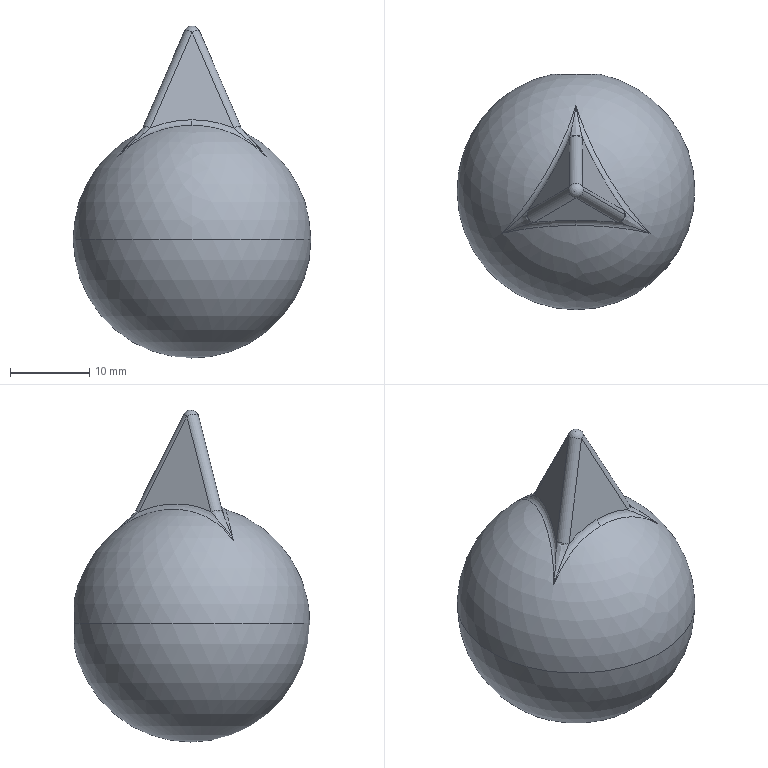Part | SolidWorks | features Fillet 2, Blend 1, ICE 1, Revolution 1 | 1 solid | 20 faces | box 30 x 29.697 x 41.877 mm | volume 14099 mm3 | cylinder 6 | torus 4 | plane 4 | sphere 3 | spline 3 | commonest cylinder face diameters 2 x4 6 x2
STEP:
#1=CARTESIAN_POINT('',(-3.,14.697,0.));
#2=VERTEX_POINT('',#1);
#3=CARTESIAN_POINT('',(0.,14.697,3.));
#4=VERTEX_POINT('',#3);
#5=CARTESIAN_POINT('',(0.,14.697,0.));
#6=DIRECTION('',(0.,1.,0.));
#7=DIRECTION('',(0.,0.,-1.));
#8=AXIS2_PLACEMENT_3D('',#5,#6,#7);
#9=CIRCLE('',#8,3.);
#10=EDGE_CURVE('',#2,#4,#9,.T.);
#11=ORIENTED_EDGE('',*,*,#10,.T.);
#12=CARTESIAN_POINT('',(0.,0.,3.));
#13=VERTEX_POINT('',#12);
#14=CARTESIAN_POINT('',(0.,26.,3.));
#15=DIRECTION('',(0.,-1.,0.));
#16=VECTOR('',#15,1000.);
#17=LINE('',#14,#16);
#18=EDGE_CURVE('',#4,#13,#17,.T.);
#19=ORIENTED_EDGE('',*,*,#18,.T.);
#20=CARTESIAN_POINT('',(0.,0.,-3.));
#21=VERTEX_POINT('',#20);
#22=CARTESIAN_POINT('',(0.,0.,0.));
#23=DIRECTION('',(0.,1.,0.));
#24=DIRECTION('',(0.,0.,1.));
#25=AXIS2_PLACEMENT_3D('',#22,#23,#24);
#26=CIRCLE('',#25,3.);
#27=EDGE_CURVE('',#21,#13,#26,.T.);
#28=ORIENTED_EDGE('',*,*,#27,.F.);
#29=CARTESIAN_POINT('',(0.,14.697,-3.));
#30=VERTEX_POINT('',#29);
#31=CARTESIAN_POINT('',(0.,26.,-3.));
#32=DIRECTION('',(0.,-1.,0.));
#33=VECTOR('',#32,1000.);
#34=LINE('',#31,#33);
#35=EDGE_CURVE('',#30,#21,#34,.T.);
#36=ORIENTED_EDGE('',*,*,#35,.F.);
#37=CARTESIAN_POINT('',(0.,14.697,0.));
#38=DIRECTION('',(0.,1.,0.));
#39=DIRECTION('',(0.,0.,-1.));
#40=AXIS2_PLACEMENT_3D('',#37,#38,#39);
#41=CIRCLE('',#40,3.);
#42=EDGE_CURVE('',#30,#2,#41,.T.);
#43=ORIENTED_EDGE('',*,*,#42,.T.);
#44=EDGE_LOOP('',(#11,#19,#28,#36,#43));
#45=FACE_OUTER_BOUND('',#44,.T.);
#46=CARTESIAN_POINT('',(0.,26.,0.));
#47=DIRECTION('',(0.,-1.,0.));
#48=DIRECTION('',(0.,0.,-1.));
#49=AXIS2_PLACEMENT_3D('',#46,#47,#48);
#50=CYLINDRICAL_SURFACE('',#49,3.);
#51=ADVANCED_FACE('',(#45),#50,.F.);
#52=CARTESIAN_POINT('',(5.23,-3.989,14.042));
#53=VERTEX_POINT('',#52);
#54=CARTESIAN_POINT('',(6.147,-3.019,14.197));
#55=VERTEX_POINT('',#54);
#56=CARTESIAN_POINT('',(5.23,-3.019,13.8));
#57=DIRECTION('',(-0.3873,0.2236,0.8944));
#58=DIRECTION('',(0.9177,0.,0.3974));
#59=AXIS2_PLACEMENT_3D('',#56,#57,#58);
#60=CIRCLE('',#59,1.);
#61=EDGE_CURVE('',#53,#55,#60,.T.);
#62=ORIENTED_EDGE('',*,*,#61,.T.);
#63=CARTESIAN_POINT('',(0.9177,0.,26.274));
#64=VERTEX_POINT('',#63);
#65=CARTESIAN_POINT('',(9.882,-5.175,5.573));
#66=DIRECTION('',(-0.3873,0.2236,0.8944));
#67=VECTOR('',#66,1000.);
#68=LINE('',#65,#67);
#69=EDGE_CURVE('',#55,#64,#68,.T.);
#70=ORIENTED_EDGE('',*,*,#69,.T.);
#71=CARTESIAN_POINT('',(0.,-0.9701,26.119));
#72=VERTEX_POINT('',#71);
#73=CARTESIAN_POINT('',(0.,0.,25.877));
#74=DIRECTION('',(-0.3873,0.2236,0.8944));
#75=DIRECTION('',(0.9177,0.,0.3974));
#76=AXIS2_PLACEMENT_3D('',#73,#74,#75);
#77=CIRCLE('',#76,1.);
#78=EDGE_CURVE('',#72,#64,#77,.T.);
#79=ORIENTED_EDGE('',*,*,#78,.F.);
#80=CARTESIAN_POINT('',(8.964,-6.146,5.418));
#81=DIRECTION('',(-0.3873,0.2236,0.8944));
#82=VECTOR('',#81,1000.);
#83=LINE('',#80,#82);
#84=EDGE_CURVE('',#53,#72,#83,.T.);
#85=ORIENTED_EDGE('',*,*,#84,.F.);
#86=EDGE_LOOP('',(#62,#70,#79,#85));
#87=FACE_OUTER_BOUND('',#86,.T.);
#88=CARTESIAN_POINT('',(8.964,-5.175,5.175));
#89=DIRECTION('',(-0.3873,0.2236,0.8944));
#90=DIRECTION('',(0.9177,0.,0.3974));
#91=AXIS2_PLACEMENT_3D('',#88,#89,#90);
#92=CYLINDRICAL_SURFACE('',#91,1.);
#93=ADVANCED_FACE('',(#87),#92,.T.);
#94=CARTESIAN_POINT('',(0.,-3.738,15.049));
#95=VERTEX_POINT('',#94);
#96=CARTESIAN_POINT('',(0.,-7.059,1.765));
#97=DIRECTION('',(0.,0.9701,-0.2425));
#98=DIRECTION('',(0.,0.2425,0.9701));
#99=AXIS2_PLACEMENT_3D('',#96,#97,#98);
#100=CIRCLE('',#99,13.693);
#101=EDGE_CURVE('',#95,#53,#100,.T.);
#102=ORIENTED_EDGE('',*,*,#101,.F.);
#103=CARTESIAN_POINT('',(0.,-4.414,14.336));
#104=VERTEX_POINT('',#103);
#105=CARTESIAN_POINT('',(0.,-4.708,15.292));
#106=DIRECTION('',(-1.,0.,0.));
#107=DIRECTION('',(0.,-1.,0.));
#108=AXIS2_PLACEMENT_3D('',#105,#106,#107);
#109=CIRCLE('',#108,1.);
#110=EDGE_CURVE('',#95,#104,#109,.T.);
#111=ORIENTED_EDGE('',*,*,#110,.T.);
#112=CARTESIAN_POINT('',(9.336,-5.39,10.43));
#113=VERTEX_POINT('',#112);
#114=CARTESIAN_POINT('',(0.,-7.527,1.882));
#115=DIRECTION('',(0.,-0.9701,0.2425));
#116=DIRECTION('',(0.,0.2425,0.9701));
#117=AXIS2_PLACEMENT_3D('',#114,#115,#116);
#118=CIRCLE('',#117,12.837);
#119=EDGE_CURVE('',#113,#104,#118,.T.);
#120=ORIENTED_EDGE('',*,*,#119,.F.);
#121=CARTESIAN_POINT('',(9.336,-5.39,10.43));
#122=CARTESIAN_POINT('',(8.724,-5.147,11.103));
#123=CARTESIAN_POINT('',(8.051,-4.9,11.718));
#124=CARTESIAN_POINT('',(6.993,-4.539,12.584));
#125=CARTESIAN_POINT('',(6.633,-4.42,12.863));
#126=CARTESIAN_POINT('',(6.092,-4.248,13.285));
#127=CARTESIAN_POINT('',(5.912,-4.192,13.426));
#128=CARTESIAN_POINT('',(5.56,-4.085,13.719));
#129=CARTESIAN_POINT('',(5.385,-4.033,13.87));
#130=CARTESIAN_POINT('',(5.23,-3.989,14.042));
#131=B_SPLINE_CURVE_WITH_KNOTS('',3,(#121,#122,#123,#124,#125,#126,#127,#128,#129,#130),.UNSPECIFIED.,.F.,.F.,(4,2,2,2,4),(-0.0000199,0.002804,0.004216,0.004922,0.005628),.UNSPECIFIED.);
#132=EDGE_CURVE('',#113,#53,#131,.T.);
#133=ORIENTED_EDGE('',*,*,#132,.T.);
#134=EDGE_LOOP('',(#102,#111,#120,#133));
#135=FACE_OUTER_BOUND('',#134,.T.);
#136=CARTESIAN_POINT('',(0.,-8.029,2.007));
#137=DIRECTION('',(0.,0.9701,-0.2425));
#138=DIRECTION('',(0.,0.2425,0.9701));
#139=AXIS2_PLACEMENT_3D('',#136,#137,#138);
#140=TOROIDAL_SURFACE('',#139,13.693,1.);
#141=ADVANCED_FACE('',(#135),#140,.F.);
#142=CARTESIAN_POINT('',(0.,-15.,0.));
#143=VERTEX_POINT('',#142);
#144=CARTESIAN_POINT('',(3.,14.697,0.));
#145=VERTEX_POINT('',#144);
#146=CARTESIAN_POINT('',(0.,0.,0.));
#147=DIRECTION('',(0.,0.,1.));
#148=DIRECTION('',(1.,0.,0.));
#149=AXIS2_PLACEMENT_3D('',#146,#147,#148);
#150=CIRCLE('',#149,15.);
#151=EDGE_CURVE('',#143,#145,#150,.T.);
#152=ORIENTED_EDGE('',*,*,#151,.F.);
#153=CARTESIAN_POINT('',(0.,0.,0.));
#154=DIRECTION('',(0.,0.,-1.));
#155=DIRECTION('',(-1.,0.,0.));
#156=AXIS2_PLACEMENT_3D('',#153,#154,#155);
#157=CIRCLE('',#156,15.);
#158=EDGE_CURVE('',#143,#2,#157,.T.);
#159=ORIENTED_EDGE('',*,*,#158,.T.);
#160=ORIENTED_EDGE('',*,*,#42,.F.);
#161=CARTESIAN_POINT('',(0.,14.697,0.));
#162=DIRECTION('',(0.,1.,0.));
#163=DIRECTION('',(0.,0.,-1.));
#164=AXIS2_PLACEMENT_3D('',#161,#162,#163);
#165=CIRCLE('',#164,3.);
#166=EDGE_CURVE('',#145,#30,#165,.T.);
#167=ORIENTED_EDGE('',*,*,#166,.F.);
#168=EDGE_LOOP('',(#152,#159,#160,#167));
#169=FACE_OUTER_BOUND('',#168,.T.);
#170=CARTESIAN_POINT('',(0.,0.,0.));
#171=DIRECTION('',(0.,0.,-1.));
#172=DIRECTION('',(1.,0.,0.));
#173=AXIS2_PLACEMENT_3D('',#170,#171,#172);
#174=SPHERICAL_SURFACE('',#173,15.);
#175=ADVANCED_FACE('',(#169),#174,.T.);
#176=ORIENTED_EDGE('',*,*,#158,.F.);
#177=ORIENTED_EDGE('',*,*,#151,.T.);
#178=CARTESIAN_POINT('',(0.,14.697,0.));
#179=DIRECTION('',(0.,1.,0.));
#180=DIRECTION('',(0.,0.,-1.));
#181=AXIS2_PLACEMENT_3D('',#178,#179,#180);
#182=CIRCLE('',#181,3.);
#183=EDGE_CURVE('',#4,#145,#182,.T.);
#184=ORIENTED_EDGE('',*,*,#183,.F.);
#185=ORIENTED_EDGE('',*,*,#10,.F.);
#186=EDGE_LOOP('',(#176,#177,#184,#185));
#187=FACE_OUTER_BOUND('',#186,.T.);
#188=CARTESIAN_POINT('',(-9.336,-5.39,10.43));
#189=VERTEX_POINT('',#188);
#190=CARTESIAN_POINT('',(0.,10.78,10.43));
#191=VERTEX_POINT('',#190);
#192=CARTESIAN_POINT('',(-6.519,3.764,1.882));
#193=DIRECTION('',(-0.8402,0.4851,0.2425));
#194=DIRECTION('',(0.5,0.866,0.));
#195=AXIS2_PLACEMENT_3D('',#192,#193,#194);
#196=CIRCLE('',#195,12.837);
#197=EDGE_CURVE('',#189,#191,#196,.T.);
#198=ORIENTED_EDGE('',*,*,#197,.T.);
#199=CARTESIAN_POINT('',(6.519,3.764,1.882));
#200=DIRECTION('',(0.8402,0.4851,0.2425));
#201=DIRECTION('',(0.5,-0.866,0.));
#202=AXIS2_PLACEMENT_3D('',#199,#200,#201);
#203=CIRCLE('',#202,12.837);
#204=EDGE_CURVE('',#191,#113,#203,.T.);
#205=ORIENTED_EDGE('',*,*,#204,.T.);
#206=ORIENTED_EDGE('',*,*,#119,.T.);
#207=CARTESIAN_POINT('',(0.,-7.527,1.882));
#208=DIRECTION('',(0.,-0.9701,0.2425));
#209=DIRECTION('',(0.,0.2425,0.9701));
#210=AXIS2_PLACEMENT_3D('',#207,#208,#209);
#211=CIRCLE('',#210,12.837);
#212=EDGE_CURVE('',#104,#189,#211,.T.);
#213=ORIENTED_EDGE('',*,*,#212,.T.);
#214=EDGE_LOOP('',(#198,#205,#206,#213));
#215=FACE_BOUND('',#214,.T.);
#216=CARTESIAN_POINT('',(0.,0.,0.));
#217=DIRECTION('',(0.,0.,-1.));
#218=DIRECTION('',(1.,0.,0.));
#219=AXIS2_PLACEMENT_3D('',#216,#217,#218);
#220=SPHERICAL_SURFACE('',#219,15.);
#221=ADVANCED_FACE('',(#187,#215),#220,.T.);
#222=ORIENTED_EDGE('',*,*,#84,.T.);
#223=CARTESIAN_POINT('',(-5.23,-3.989,14.042));
#224=VERTEX_POINT('',#223);
#225=CARTESIAN_POINT('',(-8.964,-6.146,5.418));
#226=DIRECTION('',(-0.3873,-0.2236,-0.8944));
#227=VECTOR('',#226,1000.);
#228=LINE('',#225,#227);
#229=EDGE_CURVE('',#72,#224,#228,.T.);
#230=ORIENTED_EDGE('',*,*,#229,.T.);
#231=CARTESIAN_POINT('',(0.,-7.059,1.765));
#232=DIRECTION('',(0.,0.9701,-0.2425));
#233=DIRECTION('',(0.,0.2425,0.9701));
#234=AXIS2_PLACEMENT_3D('',#231,#232,#233);
#235=CIRCLE('',#234,13.693);
#236=EDGE_CURVE('',#224,#95,#235,.T.);
#237=ORIENTED_EDGE('',*,*,#236,.T.);
#238=ORIENTED_EDGE('',*,*,#101,.T.);
#239=EDGE_LOOP('',(#222,#230,#237,#238));
#240=FACE_OUTER_BOUND('',#239,.T.);
#241=CARTESIAN_POINT('',(0.,-7.059,1.765));
#242=DIRECTION('',(0.,0.9701,-0.2425));
#243=DIRECTION('',(0.,0.2425,0.9701));
#244=AXIS2_PLACEMENT_3D('',#241,#242,#243);
#245=PLANE('',#244);
#246=ADVANCED_FACE('',(#240),#245,.F.);
#247=CARTESIAN_POINT('',(-0.8402,6.524,14.042));
#248=VERTEX_POINT('',#247);
#249=CARTESIAN_POINT('',(-6.07,-2.534,14.042));
#250=VERTEX_POINT('',#249);
#251=CARTESIAN_POINT('',(-6.113,3.529,1.765));
#252=DIRECTION('',(0.8402,-0.4851,-0.2425));
#253=DIRECTION('',(0.5,0.866,0.));
#254=AXIS2_PLACEMENT_3D('',#251,#252,#253);
#255=CIRCLE('',#254,13.693);
#256=EDGE_CURVE('',#248,#250,#255,.T.);
#257=ORIENTED_EDGE('',*,*,#256,.T.);
#258=CARTESIAN_POINT('',(-0.8402,0.4851,26.119));
#259=VERTEX_POINT('',#258);
#260=CARTESIAN_POINT('',(-9.804,-4.69,5.418));
#261=DIRECTION('',(0.3873,0.2236,0.8944));
#262=VECTOR('',#261,1000.);
#263=LINE('',#260,#262);
#264=EDGE_CURVE('',#250,#259,#263,.T.);
#265=ORIENTED_EDGE('',*,*,#264,.T.);
#266=CARTESIAN_POINT('',(-0.8402,10.836,5.418));
#267=DIRECTION('',(0.,0.4472,-0.8944));
#268=VECTOR('',#267,1000.);
#269=LINE('',#266,#268);
#270=EDGE_CURVE('',#259,#248,#269,.T.);
#271=ORIENTED_EDGE('',*,*,#270,.T.);
#272=EDGE_LOOP('',(#257,#265,#271));
#273=FACE_OUTER_BOUND('',#272,.T.);
#274=CARTESIAN_POINT('',(-6.113,3.529,1.765));
#275=DIRECTION('',(0.8402,-0.4851,-0.2425));
#276=DIRECTION('',(0.5,0.866,0.));
#277=AXIS2_PLACEMENT_3D('',#274,#275,#276);
#278=PLANE('',#277);
#279=ADVANCED_FACE('',(#273),#278,.F.);
#280=CARTESIAN_POINT('',(0.8402,6.524,14.042));
#281=VERTEX_POINT('',#280);
#282=CARTESIAN_POINT('',(0.8402,0.4851,26.119));
#283=VERTEX_POINT('',#282);
#284=CARTESIAN_POINT('',(0.8402,10.836,5.418));
#285=DIRECTION('',(0.,-0.4472,0.8944));
#286=VECTOR('',#285,1000.);
#287=LINE('',#284,#286);
#288=EDGE_CURVE('',#281,#283,#287,.T.);
#289=ORIENTED_EDGE('',*,*,#288,.T.);
#290=CARTESIAN_POINT('',(6.07,-2.534,14.042));
#291=VERTEX_POINT('',#290);
#292=CARTESIAN_POINT('',(9.804,-4.69,5.418));
#293=DIRECTION('',(0.3873,-0.2236,-0.8944));
#294=VECTOR('',#293,1000.);
#295=LINE('',#292,#294);
#296=EDGE_CURVE('',#283,#291,#295,.T.);
#297=ORIENTED_EDGE('',*,*,#296,.T.);
#298=CARTESIAN_POINT('',(6.113,3.529,1.765));
#299=DIRECTION('',(-0.8402,-0.4851,-0.2425));
#300=DIRECTION('',(0.5,-0.866,0.));
#301=AXIS2_PLACEMENT_3D('',#298,#299,#300);
#302=CIRCLE('',#301,13.693);
#303=EDGE_CURVE('',#291,#281,#302,.T.);
#304=ORIENTED_EDGE('',*,*,#303,.T.);
#305=EDGE_LOOP('',(#289,#297,#304));
#306=FACE_OUTER_BOUND('',#305,.T.);
#307=CARTESIAN_POINT('',(6.113,3.529,1.765));
#308=DIRECTION('',(-0.8402,-0.4851,-0.2425));
#309=DIRECTION('',(0.5,-0.866,0.));
#310=AXIS2_PLACEMENT_3D('',#307,#308,#309);
#311=PLANE('',#310);
#312=ADVANCED_FACE('',(#306),#311,.F.);
#313=ORIENTED_EDGE('',*,*,#110,.F.);
#314=ORIENTED_EDGE('',*,*,#236,.F.);
#315=CARTESIAN_POINT('',(-5.23,-3.989,14.042));
#316=CARTESIAN_POINT('',(-5.385,-4.033,13.87));
#317=CARTESIAN_POINT('',(-5.56,-4.085,13.719));
#318=CARTESIAN_POINT('',(-5.912,-4.192,13.426));
#319=CARTESIAN_POINT('',(-6.092,-4.248,13.285));
#320=CARTESIAN_POINT('',(-6.633,-4.42,12.863));
#321=CARTESIAN_POINT('',(-6.993,-4.539,12.584));
#322=CARTESIAN_POINT('',(-8.051,-4.9,11.718));
#323=CARTESIAN_POINT('',(-8.723,-5.147,11.104));
#324=CARTESIAN_POINT('',(-9.336,-5.39,10.43));
#325=B_SPLINE_CURVE_WITH_KNOTS('',3,(#315,#316,#317,#318,#319,#320,#321,#322,#323,#324),.UNSPECIFIED.,.F.,.F.,(4,2,2,2,4),(0.,0.0007073,0.001415,0.002829,0.005658),.UNSPECIFIED.);
#326=EDGE_CURVE('',#224,#189,#325,.T.);
#327=ORIENTED_EDGE('',*,*,#326,.T.);
#328=ORIENTED_EDGE('',*,*,#212,.F.);
#329=EDGE_LOOP('',(#313,#314,#327,#328));
#330=FACE_OUTER_BOUND('',#329,.T.);
#331=CARTESIAN_POINT('',(0.,-8.029,2.007));
#332=DIRECTION('',(0.,0.9701,-0.2425));
#333=DIRECTION('',(0.,0.2425,0.9701));
#334=AXIS2_PLACEMENT_3D('',#331,#332,#333);
#335=TOROIDAL_SURFACE('',#334,13.693,1.);
#336=ADVANCED_FACE('',(#330),#335,.F.);
#337=ORIENTED_EDGE('',*,*,#197,.F.);
#338=CARTESIAN_POINT('',(-9.336,-5.39,10.43));
#339=CARTESIAN_POINT('',(-8.82,-4.982,11.103));
#340=CARTESIAN_POINT('',(-8.269,-4.522,11.718));
#341=CARTESIAN_POINT('',(-7.428,-3.787,12.584));
#342=CARTESIAN_POINT('',(-7.144,-3.534,12.863));
#343=CARTESIAN_POINT('',(-6.725,-3.152,13.285));
#344=CARTESIAN_POINT('',(-6.587,-3.024,13.426));
#345=CARTESIAN_POINT('',(-6.317,-2.773,13.719));
#346=CARTESIAN_POINT('',(-6.185,-2.647,13.87));
#347=CARTESIAN_POINT('',(-6.07,-2.534,14.042));
#348=B_SPLINE_CURVE_WITH_KNOTS('',3,(#338,#339,#340,#341,#342,#343,#344,#345,#346,#347),.UNSPECIFIED.,.F.,.F.,(4,2,2,2,4),(-0.00002565,0.002798,0.00421,0.004916,0.005622),.UNSPECIFIED.);
#349=EDGE_CURVE('',#189,#250,#348,.T.);
#350=ORIENTED_EDGE('',*,*,#349,.T.);
#351=ORIENTED_EDGE('',*,*,#256,.F.);
#352=CARTESIAN_POINT('',(-0.8402,6.524,14.042));
#353=CARTESIAN_POINT('',(-0.7998,6.68,13.87));
#354=CARTESIAN_POINT('',(-0.7574,6.857,13.719));
#355=CARTESIAN_POINT('',(-0.6741,7.216,13.426));
#356=CARTESIAN_POINT('',(-0.6328,7.4,13.285));
#357=CARTESIAN_POINT('',(-0.5114,7.954,12.863));
#358=CARTESIAN_POINT('',(-0.4341,8.326,12.584));
#359=CARTESIAN_POINT('',(-0.218,9.423,11.718));
#360=CARTESIAN_POINT('',(-0.09559,10.128,11.104));
#361=CARTESIAN_POINT('',(0.,10.78,10.43));
#362=B_SPLINE_CURVE_WITH_KNOTS('',3,(#352,#353,#354,#355,#356,#357,#358,#359,#360,#361),.UNSPECIFIED.,.F.,.F.,(4,2,2,2,4),(0.,0.0007073,0.001415,0.002829,0.005658),.UNSPECIFIED.);
#363=EDGE_CURVE('',#248,#191,#362,.T.);
#364=ORIENTED_EDGE('',*,*,#363,.T.);
#365=EDGE_LOOP('',(#337,#350,#351,#364));
#366=FACE_OUTER_BOUND('',#365,.T.);
#367=CARTESIAN_POINT('',(-6.953,4.014,2.007));
#368=DIRECTION('',(0.8402,-0.4851,-0.2425));
#369=DIRECTION('',(0.5,0.866,0.));
#370=AXIS2_PLACEMENT_3D('',#367,#368,#369);
#371=TOROIDAL_SURFACE('',#370,13.693,1.);
#372=ADVANCED_FACE('',(#366),#371,.F.);
#373=ORIENTED_EDGE('',*,*,#303,.F.);
#374=CARTESIAN_POINT('',(6.07,-2.534,14.042));
#375=CARTESIAN_POINT('',(6.185,-2.647,13.87));
#376=CARTESIAN_POINT('',(6.317,-2.773,13.719));
#377=CARTESIAN_POINT('',(6.587,-3.024,13.426));
#378=CARTESIAN_POINT('',(6.725,-3.152,13.285));
#379=CARTESIAN_POINT('',(7.144,-3.534,12.863));
#380=CARTESIAN_POINT('',(7.428,-3.787,12.584));
#381=CARTESIAN_POINT('',(8.269,-4.522,11.718));
#382=CARTESIAN_POINT('',(8.819,-4.981,11.104));
#383=CARTESIAN_POINT('',(9.336,-5.39,10.43));
#384=B_SPLINE_CURVE_WITH_KNOTS('',3,(#374,#375,#376,#377,#378,#379,#380,#381,#382,#383),.UNSPECIFIED.,.F.,.F.,(4,2,2,2,4),(0.,0.0007073,0.001415,0.002829,0.005658),.UNSPECIFIED.);
#385=EDGE_CURVE('',#291,#113,#384,.T.);
#386=ORIENTED_EDGE('',*,*,#385,.T.);
#387=ORIENTED_EDGE('',*,*,#204,.F.);
#388=CARTESIAN_POINT('',(0.,10.78,10.43));
#389=CARTESIAN_POINT('',(0.09546,10.129,11.103));
#390=CARTESIAN_POINT('',(0.218,9.423,11.718));
#391=CARTESIAN_POINT('',(0.4341,8.326,12.584));
#392=CARTESIAN_POINT('',(0.5114,7.954,12.863));
#393=CARTESIAN_POINT('',(0.6328,7.4,13.285));
#394=CARTESIAN_POINT('',(0.6741,7.216,13.426));
#395=CARTESIAN_POINT('',(0.7574,6.857,13.719));
#396=CARTESIAN_POINT('',(0.7998,6.68,13.87));
#397=CARTESIAN_POINT('',(0.8402,6.524,14.042));
#398=B_SPLINE_CURVE_WITH_KNOTS('',3,(#388,#389,#390,#391,#392,#393,#394,#395,#396,#397),.UNSPECIFIED.,.F.,.F.,(4,2,2,2,4),(-0.00002565,0.002798,0.00421,0.004916,0.005622),.UNSPECIFIED.);
#399=EDGE_CURVE('',#191,#281,#398,.T.);
#400=ORIENTED_EDGE('',*,*,#399,.T.);
#401=EDGE_LOOP('',(#373,#386,#387,#400));
#402=FACE_OUTER_BOUND('',#401,.T.);
#403=CARTESIAN_POINT('',(6.953,4.014,2.007));
#404=DIRECTION('',(-0.8402,-0.4851,-0.2425));
#405=DIRECTION('',(0.5,-0.866,0.));
#406=AXIS2_PLACEMENT_3D('',#403,#404,#405);
#407=TOROIDAL_SURFACE('',#406,13.693,1.);
#408=ADVANCED_FACE('',(#402),#407,.F.);
#409=ORIENTED_EDGE('',*,*,#399,.F.);
#410=ORIENTED_EDGE('',*,*,#363,.F.);
#411=CARTESIAN_POINT('',(0.,6.039,13.8));
#412=DIRECTION('',(0.,-0.4472,0.8944));
#413=DIRECTION('',(0.,-0.8944,-0.4472));
#414=AXIS2_PLACEMENT_3D('',#411,#412,#413);
#415=CIRCLE('',#414,1.);
#416=EDGE_CURVE('',#281,#248,#415,.T.);
#417=ORIENTED_EDGE('',*,*,#416,.F.);
#418=EDGE_LOOP('',(#409,#410,#417));
#419=FACE_OUTER_BOUND('',#418,.T.);
#420=CARTESIAN_POINT('',(0.,10.78,10.43));
#421=CARTESIAN_POINT('',(0.,10.78,10.43));
#422=CARTESIAN_POINT('',(0.,10.78,10.43));
#423=CARTESIAN_POINT('',(-0.05112,10.431,10.792));
#424=CARTESIAN_POINT('',(0.,10.431,10.792));
#425=CARTESIAN_POINT('',(0.05112,10.431,10.792));
#426=CARTESIAN_POINT('',(-0.1096,10.069,11.133));
#427=CARTESIAN_POINT('',(0.,10.07,11.143));
#428=CARTESIAN_POINT('',(0.1096,10.069,11.133));
#429=CARTESIAN_POINT('',(-0.2387,9.331,11.782));
#430=CARTESIAN_POINT('',(0.,9.363,11.826));
#431=CARTESIAN_POINT('',(0.2387,9.331,11.782));
#432=CARTESIAN_POINT('',(-0.3094,8.955,12.089));
#433=CARTESIAN_POINT('',(0.,9.005,12.17));
#434=CARTESIAN_POINT('',(0.3094,8.955,12.089));
#435=CARTESIAN_POINT('',(-0.4212,8.394,12.528));
#436=CARTESIAN_POINT('',(0.,8.52,12.675));
#437=CARTESIAN_POINT('',(0.4212,8.394,12.528));
#438=CARTESIAN_POINT('',(-0.4595,8.207,12.671));
#439=CARTESIAN_POINT('',(0.,8.361,12.85));
#440=CARTESIAN_POINT('',(0.4595,8.207,12.671));
#441=CARTESIAN_POINT('',(-0.5372,7.838,12.952));
#442=CARTESIAN_POINT('',(0.,8.066,13.203));
#443=CARTESIAN_POINT('',(0.5372,7.838,12.952));
#444=CARTESIAN_POINT('',(-0.5766,7.655,13.09));
#445=CARTESIAN_POINT('',(0.,7.929,13.386));
#446=CARTESIAN_POINT('',(0.5766,7.655,13.09));
#447=CARTESIAN_POINT('',(-0.6553,7.3,13.362));
#448=CARTESIAN_POINT('',(0.,7.703,13.757));
#449=CARTESIAN_POINT('',(0.6553,7.3,13.362));
#450=CARTESIAN_POINT('',(-0.6945,7.127,13.496));
#451=CARTESIAN_POINT('',(0.,7.614,13.951));
#452=CARTESIAN_POINT('',(0.6945,7.127,13.496));
#453=CARTESIAN_POINT('',(-0.7515,6.884,13.699));
#454=CARTESIAN_POINT('',(0.,7.557,14.225));
#455=CARTESIAN_POINT('',(0.7515,6.884,13.699));
#456=CARTESIAN_POINT('',(-0.7702,6.805,13.767));
#457=CARTESIAN_POINT('',(0.,7.552,14.319));
#458=CARTESIAN_POINT('',(0.7702,6.805,13.767));
#459=CARTESIAN_POINT('',(-0.8065,6.656,13.904));
#460=CARTESIAN_POINT('',(0.,7.583,14.492));
#461=CARTESIAN_POINT('',(0.8065,6.656,13.904));
#462=CARTESIAN_POINT('',(-0.8239,6.587,13.973));
#463=CARTESIAN_POINT('',(0.,7.622,14.571));
#464=CARTESIAN_POINT('',(0.8239,6.587,13.973));
#465=CARTESIAN_POINT('',(-0.8402,6.524,14.042));
#466=CARTESIAN_POINT('',(0.,7.688,14.624));
#467=CARTESIAN_POINT('',(0.8402,6.524,14.042));
#468=(BOUNDED_SURFACE()B_SPLINE_SURFACE(3,2,((#420,#421,#422),(#423,#424,#425),(#426,#427,#428),(#429,#430,#431),(#432,#433,#434),(#435,#436,#437),(#438,#439,#440),(#441,#442,#443),(#444,#445,#446),(#447,#448,#449),(#450,#451,#452),(#453,#454,#455),(#456,#457,#458),(#459,#460,#461),(#462,#463,#464),(#465,#466,#467)),.UNSPECIFIED.,.F.,.F.,.T.)B_SPLINE_SURFACE_WITH_KNOTS((4,2,2,2,2,2,2,4),(3,3),(-0.00001368,0.001421,0.002855,0.003572,0.004289,0.005006,0.005365,0.005723),(0.,1.),.UNSPECIFIED.)GEOMETRIC_REPRESENTATION_ITEM()RATIONAL_B_SPLINE_SURFACE(((1.,1.,1.),(1.,1.,1.),(1.,0.9961,1.),(1.,0.9733,1.),(1.,0.9544,1.),(1.,0.9078,1.),(1.,0.8893,1.),(1.,0.8447,1.),(1.,0.8185,1.),(1.,0.7571,1.),(1.,0.7217,1.),(1.,0.6603,1.),(1.,0.6385,1.),(1.,0.592,1.),(1.,0.5675,1.),(1.,0.5423,1.)))REPRESENTATION_ITEM('')SURFACE());
#469=ADVANCED_FACE('',(#419),#468,.T.);
#470=ORIENTED_EDGE('',*,*,#132,.F.);
#471=ORIENTED_EDGE('',*,*,#385,.F.);
#472=CARTESIAN_POINT('',(5.23,-3.019,13.8));
#473=DIRECTION('',(-0.3873,0.2236,0.8944));
#474=DIRECTION('',(0.9177,0.,0.3974));
#475=AXIS2_PLACEMENT_3D('',#472,#473,#474);
#476=CIRCLE('',#475,1.);
#477=EDGE_CURVE('',#55,#291,#476,.T.);
#478=ORIENTED_EDGE('',*,*,#477,.F.);
#479=ORIENTED_EDGE('',*,*,#61,.F.);
#480=EDGE_LOOP('',(#470,#471,#478,#479));
#481=FACE_OUTER_BOUND('',#480,.T.);
#482=CARTESIAN_POINT('',(9.336,-5.39,10.43));
#483=CARTESIAN_POINT('',(9.336,-5.39,10.43));
#484=CARTESIAN_POINT('',(9.336,-5.39,10.43));
#485=CARTESIAN_POINT('',(9.059,-5.171,10.792));
#486=CARTESIAN_POINT('',(9.033,-5.215,10.792));
#487=CARTESIAN_POINT('',(9.008,-5.26,10.792));
#488=CARTESIAN_POINT('',(8.774,-4.939,11.133));
#489=CARTESIAN_POINT('',(8.721,-5.035,11.143));
#490=CARTESIAN_POINT('',(8.665,-5.129,11.133));
#491=CARTESIAN_POINT('',(8.2,-4.459,11.782));
#492=CARTESIAN_POINT('',(8.109,-4.682,11.826));
#493=CARTESIAN_POINT('',(7.962,-4.872,11.782));
#494=CARTESIAN_POINT('',(7.91,-4.21,12.089));
#495=CARTESIAN_POINT('',(7.799,-4.503,12.17));
#496=CARTESIAN_POINT('',(7.601,-4.746,12.089));
#497=CARTESIAN_POINT('',(7.48,-3.832,12.528));
#498=CARTESIAN_POINT('',(7.379,-4.26,12.675));
#499=CARTESIAN_POINT('',(7.059,-4.562,12.528));
#500=CARTESIAN_POINT('',(7.337,-3.706,12.671));
#501=CARTESIAN_POINT('',(7.241,-4.18,12.85));
#502=CARTESIAN_POINT('',(6.878,-4.502,12.671));
#503=CARTESIAN_POINT('',(7.056,-3.454,12.952));
#504=CARTESIAN_POINT('',(6.985,-4.033,13.203));
#505=CARTESIAN_POINT('',(6.519,-4.384,12.952));
#506=CARTESIAN_POINT('',(6.918,-3.328,13.09));
#507=CARTESIAN_POINT('',(6.867,-3.965,13.386));
#508=CARTESIAN_POINT('',(6.341,-4.327,13.09));
#509=CARTESIAN_POINT('',(6.65,-3.083,13.362));
#510=CARTESIAN_POINT('',(6.671,-3.851,13.757));
#511=CARTESIAN_POINT('',(5.994,-4.217,13.362));
#512=CARTESIAN_POINT('',(6.52,-2.962,13.496));
#513=CARTESIAN_POINT('',(6.594,-3.807,13.951));
#514=CARTESIAN_POINT('',(5.825,-4.165,13.496));
#515=CARTESIAN_POINT('',(6.337,-2.791,13.699));
#516=CARTESIAN_POINT('',(6.545,-3.779,14.225));
#517=CARTESIAN_POINT('',(5.586,-4.093,13.699));
#518=CARTESIAN_POINT('',(6.279,-2.736,13.767));
#519=CARTESIAN_POINT('',(6.541,-3.776,14.319));
#520=CARTESIAN_POINT('',(5.509,-4.07,13.767));
#521=CARTESIAN_POINT('',(6.168,-2.63,13.904));
#522=CARTESIAN_POINT('',(6.567,-3.792,14.492));
#523=CARTESIAN_POINT('',(5.361,-4.027,13.904));
#524=CARTESIAN_POINT('',(6.116,-2.58,13.973));
#525=CARTESIAN_POINT('',(6.601,-3.811,14.571));
#526=CARTESIAN_POINT('',(5.292,-4.007,13.973));
#527=CARTESIAN_POINT('',(6.07,-2.534,14.042));
#528=CARTESIAN_POINT('',(6.658,-3.844,14.624));
#529=CARTESIAN_POINT('',(5.23,-3.989,14.042));
#530=(BOUNDED_SURFACE()B_SPLINE_SURFACE(3,2,((#482,#483,#484),(#485,#486,#487),(#488,#489,#490),(#491,#492,#493),(#494,#495,#496),(#497,#498,#499),(#500,#501,#502),(#503,#504,#505),(#506,#507,#508),(#509,#510,#511),(#512,#513,#514),(#515,#516,#517),(#518,#519,#520),(#521,#522,#523),(#524,#525,#526),(#527,#528,#529)),.UNSPECIFIED.,.F.,.F.,.F.)B_SPLINE_SURFACE_WITH_KNOTS((4,2,2,2,2,2,2,4),(3,3),(-0.00001368,0.001421,0.002855,0.003572,0.004289,0.005006,0.005365,0.005723),(0.,1.),.UNSPECIFIED.)GEOMETRIC_REPRESENTATION_ITEM()RATIONAL_B_SPLINE_SURFACE(((1.,1.,1.),(1.,1.,1.),(1.,0.9961,1.),(1.,0.9733,1.),(1.,0.9544,1.),(1.,0.9078,1.),(1.,0.8893,1.),(1.,0.8447,1.),(1.,0.8185,1.),(1.,0.7571,1.),(1.,0.7217,1.),(1.,0.6603,1.),(1.,0.6385,1.),(1.,0.592,1.),(1.,0.5675,1.),(1.,0.5423,1.)))REPRESENTATION_ITEM('')SURFACE());
#531=ADVANCED_FACE('',(#481),#530,.T.);
#532=ORIENTED_EDGE('',*,*,#416,.T.);
#533=ORIENTED_EDGE('',*,*,#270,.F.);
#534=CARTESIAN_POINT('',(0.,0.,25.877));
#535=DIRECTION('',(0.,-0.4472,0.8944));
#536=DIRECTION('',(0.,-0.8944,-0.4472));
#537=AXIS2_PLACEMENT_3D('',#534,#535,#536);
#538=CIRCLE('',#537,1.);
#539=EDGE_CURVE('',#283,#259,#538,.T.);
#540=ORIENTED_EDGE('',*,*,#539,.F.);
#541=ORIENTED_EDGE('',*,*,#288,.F.);
#542=EDGE_LOOP('',(#532,#533,#540,#541));
#543=FACE_OUTER_BOUND('',#542,.T.);
#544=CARTESIAN_POINT('',(0.,10.351,5.175));
#545=DIRECTION('',(0.,-0.4472,0.8944));
#546=DIRECTION('',(0.,-0.8944,-0.4472));
#547=AXIS2_PLACEMENT_3D('',#544,#545,#546);
#548=CYLINDRICAL_SURFACE('',#547,1.);
#549=ADVANCED_FACE('',(#543),#548,.T.);
#550=ORIENTED_EDGE('',*,*,#69,.F.);
#551=ORIENTED_EDGE('',*,*,#477,.T.);
#552=ORIENTED_EDGE('',*,*,#296,.F.);
#553=CARTESIAN_POINT('',(0.,0.,25.877));
#554=DIRECTION('',(-0.3873,0.2236,0.8944));
#555=DIRECTION('',(0.9177,0.,0.3974));
#556=AXIS2_PLACEMENT_3D('',#553,#554,#555);
#557=CIRCLE('',#556,1.);
#558=EDGE_CURVE('',#64,#283,#557,.T.);
#559=ORIENTED_EDGE('',*,*,#558,.F.);
#560=EDGE_LOOP('',(#550,#551,#552,#559));
#561=FACE_OUTER_BOUND('',#560,.T.);
#562=CARTESIAN_POINT('',(8.964,-5.175,5.175));
#563=DIRECTION('',(-0.3873,0.2236,0.8944));
#564=DIRECTION('',(0.9177,0.,0.3974));
#565=AXIS2_PLACEMENT_3D('',#562,#563,#564);
#566=CYLINDRICAL_SURFACE('',#565,1.);
#567=ADVANCED_FACE('',(#561),#566,.T.);
#568=ORIENTED_EDGE('',*,*,#78,.T.);
#569=ORIENTED_EDGE('',*,*,#558,.T.);
#570=ORIENTED_EDGE('',*,*,#539,.T.);
#571=CARTESIAN_POINT('',(0.,0.,25.877));
#572=DIRECTION('',(-0.3873,-0.2236,-0.8944));
#573=DIRECTION('',(0.9177,0.,-0.3974));
#574=AXIS2_PLACEMENT_3D('',#571,#572,#573);
#575=CIRCLE('',#574,1.);
#576=EDGE_CURVE('',#72,#259,#575,.T.);
#577=ORIENTED_EDGE('',*,*,#576,.F.);
#578=EDGE_LOOP('',(#568,#569,#570,#577));
#579=FACE_OUTER_BOUND('',#578,.T.);
#580=CARTESIAN_POINT('',(0.,0.,25.877));
#581=DIRECTION('',(-0.21,-0.1213,0.9701));
#582=DIRECTION('',(-0.5,0.866,0.));
#583=AXIS2_PLACEMENT_3D('',#580,#581,#582);
#584=SPHERICAL_SURFACE('',#583,1.);
#585=ADVANCED_FACE('',(#579),#584,.T.);
#586=ORIENTED_EDGE('',*,*,#576,.T.);
#587=ORIENTED_EDGE('',*,*,#264,.F.);
#588=CARTESIAN_POINT('',(-5.23,-3.019,13.8));
#589=DIRECTION('',(-0.3873,-0.2236,-0.8944));
#590=DIRECTION('',(-0.9177,0.,0.3974));
#591=AXIS2_PLACEMENT_3D('',#588,#589,#590);
#592=CIRCLE('',#591,1.);
#593=EDGE_CURVE('',#224,#250,#592,.T.);
#594=ORIENTED_EDGE('',*,*,#593,.F.);
#595=ORIENTED_EDGE('',*,*,#229,.F.);
#596=EDGE_LOOP('',(#586,#587,#594,#595));
#597=FACE_OUTER_BOUND('',#596,.T.);
#598=CARTESIAN_POINT('',(-8.964,-5.175,5.175));
#599=DIRECTION('',(0.3873,0.2236,0.8944));
#600=DIRECTION('',(0.9177,0.,-0.3974));
#601=AXIS2_PLACEMENT_3D('',#598,#599,#600);
#602=CYLINDRICAL_SURFACE('',#601,1.);
#603=ADVANCED_FACE('',(#597),#602,.T.);
#604=ORIENTED_EDGE('',*,*,#349,.F.);
#605=ORIENTED_EDGE('',*,*,#326,.F.);
#606=ORIENTED_EDGE('',*,*,#593,.T.);
#607=EDGE_LOOP('',(#604,#605,#606));
#608=FACE_OUTER_BOUND('',#607,.T.);
#609=CARTESIAN_POINT('',(-9.336,-5.39,10.43));
#610=CARTESIAN_POINT('',(-9.336,-5.39,10.43));
#611=CARTESIAN_POINT('',(-9.336,-5.39,10.43));
#612=CARTESIAN_POINT('',(-9.008,-5.26,10.792));
#613=CARTESIAN_POINT('',(-9.033,-5.215,10.792));
#614=CARTESIAN_POINT('',(-9.059,-5.171,10.792));
#615=CARTESIAN_POINT('',(-8.665,-5.129,11.133));
#616=CARTESIAN_POINT('',(-8.721,-5.035,11.143));
#617=CARTESIAN_POINT('',(-8.774,-4.939,11.133));
#618=CARTESIAN_POINT('',(-7.962,-4.872,11.782));
#619=CARTESIAN_POINT('',(-8.109,-4.682,11.826));
#620=CARTESIAN_POINT('',(-8.2,-4.459,11.782));
#621=CARTESIAN_POINT('',(-7.601,-4.746,12.089));
#622=CARTESIAN_POINT('',(-7.799,-4.503,12.17));
#623=CARTESIAN_POINT('',(-7.91,-4.21,12.089));
#624=CARTESIAN_POINT('',(-7.059,-4.562,12.528));
#625=CARTESIAN_POINT('',(-7.379,-4.26,12.675));
#626=CARTESIAN_POINT('',(-7.48,-3.832,12.528));
#627=CARTESIAN_POINT('',(-6.878,-4.502,12.671));
#628=CARTESIAN_POINT('',(-7.241,-4.18,12.85));
#629=CARTESIAN_POINT('',(-7.337,-3.706,12.671));
#630=CARTESIAN_POINT('',(-6.519,-4.384,12.952));
#631=CARTESIAN_POINT('',(-6.985,-4.033,13.203));
#632=CARTESIAN_POINT('',(-7.056,-3.454,12.952));
#633=CARTESIAN_POINT('',(-6.341,-4.327,13.09));
#634=CARTESIAN_POINT('',(-6.867,-3.965,13.386));
#635=CARTESIAN_POINT('',(-6.918,-3.328,13.09));
#636=CARTESIAN_POINT('',(-5.994,-4.217,13.362));
#637=CARTESIAN_POINT('',(-6.671,-3.851,13.757));
#638=CARTESIAN_POINT('',(-6.65,-3.083,13.362));
#639=CARTESIAN_POINT('',(-5.825,-4.165,13.496));
#640=CARTESIAN_POINT('',(-6.594,-3.807,13.951));
#641=CARTESIAN_POINT('',(-6.52,-2.962,13.496));
#642=CARTESIAN_POINT('',(-5.586,-4.093,13.699));
#643=CARTESIAN_POINT('',(-6.545,-3.779,14.225));
#644=CARTESIAN_POINT('',(-6.337,-2.791,13.699));
#645=CARTESIAN_POINT('',(-5.509,-4.07,13.767));
#646=CARTESIAN_POINT('',(-6.541,-3.776,14.319));
#647=CARTESIAN_POINT('',(-6.279,-2.736,13.767));
#648=CARTESIAN_POINT('',(-5.361,-4.027,13.904));
#649=CARTESIAN_POINT('',(-6.567,-3.792,14.492));
#650=CARTESIAN_POINT('',(-6.168,-2.63,13.904));
#651=CARTESIAN_POINT('',(-5.292,-4.007,13.973));
#652=CARTESIAN_POINT('',(-6.601,-3.811,14.571));
#653=CARTESIAN_POINT('',(-6.116,-2.58,13.973));
#654=CARTESIAN_POINT('',(-5.23,-3.989,14.042));
#655=CARTESIAN_POINT('',(-6.658,-3.844,14.624));
#656=CARTESIAN_POINT('',(-6.07,-2.534,14.042));
#657=(BOUNDED_SURFACE()B_SPLINE_SURFACE(3,2,((#609,#610,#611),(#612,#613,#614),(#615,#616,#617),(#618,#619,#620),(#621,#622,#623),(#624,#625,#626),(#627,#628,#629),(#630,#631,#632),(#633,#634,#635),(#636,#637,#638),(#639,#640,#641),(#642,#643,#644),(#645,#646,#647),(#648,#649,#650),(#651,#652,#653),(#654,#655,#656)),.UNSPECIFIED.,.F.,.F.,.T.)B_SPLINE_SURFACE_WITH_KNOTS((4,2,2,2,2,2,2,4),(3,3),(-0.00001368,0.001421,0.002855,0.003572,0.004289,0.005006,0.005365,0.005723),(0.,1.),.UNSPECIFIED.)GEOMETRIC_REPRESENTATION_ITEM()RATIONAL_B_SPLINE_SURFACE(((1.,1.,1.),(1.,1.,1.),(1.,0.9961,1.),(1.,0.9733,1.),(1.,0.9544,1.),(1.,0.9078,1.),(1.,0.8893,1.),(1.,0.8447,1.),(1.,0.8185,1.),(1.,0.7571,1.),(1.,0.7217,1.),(1.,0.6603,1.),(1.,0.6385,1.),(1.,0.592,1.),(1.,0.5675,1.),(1.,0.5423,1.)))REPRESENTATION_ITEM('')SURFACE());
#658=ADVANCED_FACE('',(#608),#657,.T.);
#659=ORIENTED_EDGE('',*,*,#18,.F.);
#660=ORIENTED_EDGE('',*,*,#183,.T.);
#661=ORIENTED_EDGE('',*,*,#166,.T.);
#662=ORIENTED_EDGE('',*,*,#35,.T.);
#663=CARTESIAN_POINT('',(0.,0.,0.));
#664=DIRECTION('',(0.,1.,0.));
#665=DIRECTION('',(0.,0.,1.));
#666=AXIS2_PLACEMENT_3D('',#663,#664,#665);
#667=CIRCLE('',#666,3.);
#668=EDGE_CURVE('',#13,#21,#667,.T.);
#669=ORIENTED_EDGE('',*,*,#668,.F.);
#670=EDGE_LOOP('',(#659,#660,#661,#662,#669));
#671=FACE_OUTER_BOUND('',#670,.T.);
#672=CARTESIAN_POINT('',(0.,26.,0.));
#673=DIRECTION('',(0.,-1.,0.));
#674=DIRECTION('',(0.,0.,-1.));
#675=AXIS2_PLACEMENT_3D('',#672,#673,#674);
#676=CYLINDRICAL_SURFACE('',#675,3.);
#677=ADVANCED_FACE('',(#671),#676,.F.);
#678=ORIENTED_EDGE('',*,*,#27,.T.);
#679=ORIENTED_EDGE('',*,*,#668,.T.);
#680=EDGE_LOOP('',(#678,#679));
#681=FACE_OUTER_BOUND('',#680,.T.);
#682=CARTESIAN_POINT('',(0.,0.,0.));
#683=DIRECTION('',(0.,1.,0.));
#684=DIRECTION('',(0.,0.,1.));
#685=AXIS2_PLACEMENT_3D('',#682,#683,#684);
#686=PLANE('',#685);
#687=ADVANCED_FACE('',(#681),#686,.T.);
#688=CLOSED_SHELL('',(#51,#93,#141,#175,#221,#246,#279,#312,#336,#372,#408,#469,#531,#549,#567,#585,#603,#658,#677,#687));
#689=MANIFOLD_SOLID_BREP('',#688);
#690=CARTESIAN_POINT('',(0.,0.,0.));
#691=DIRECTION('',(0.,0.,1.));
#692=DIRECTION('',(1.,0.,0.));
#693=AXIS2_PLACEMENT_3D('',#690,#691,#692);
#694=(LENGTH_UNIT()NAMED_UNIT(*)SI_UNIT(.MILLI.,.METRE.));
#695=UNCERTAINTY_MEASURE_WITH_UNIT(LENGTH_MEASURE(0.00001),#694,'','');
#696=(NAMED_UNIT(*)PLANE_ANGLE_UNIT()SI_UNIT($,.RADIAN.));
#697=(NAMED_UNIT(*)SI_UNIT($,.STERADIAN.)SOLID_ANGLE_UNIT());
#698=(GEOMETRIC_REPRESENTATION_CONTEXT(3)GLOBAL_UNCERTAINTY_ASSIGNED_CONTEXT((#695))GLOBAL_UNIT_ASSIGNED_CONTEXT((#694,#696,#697))REPRESENTATION_CONTEXT('',''));
#699=ADVANCED_BREP_SHAPE_REPRESENTATION('',(#689,#693),#698);